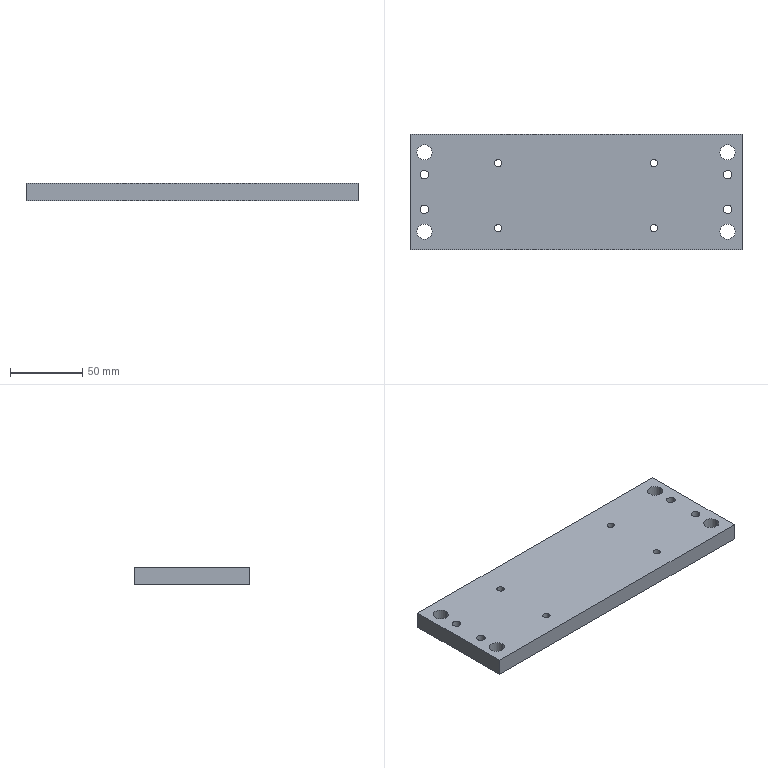Part | STEP file | PN_0023 | 1 solid | 30 faces | box 230 x 80 x 12 mm | volume 214344 mm3 | cylinder 24 | plane 6 | commonest cylinder face diameters 5 x8 6 x8 10.5 x8